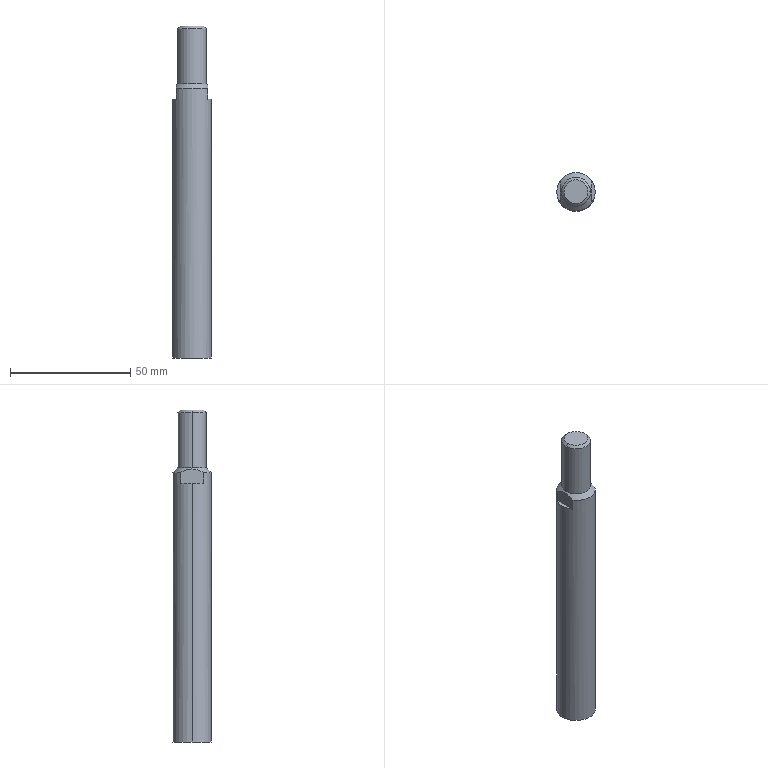Part | STEP file | 1 solid | 14 faces | box 16 x 16 x 138 mm | volume 25426 mm3 | plane 6 | cylinder 4 | cone 4 | commonest cylinder face diameters 12 x2 16 x2
STEP:
#1=CARTESIAN_POINT('',(8.,0.,-84.));
#2=VERTEX_POINT('',#1);
#3=CARTESIAN_POINT('',(-8.,0.,-84.));
#4=VERTEX_POINT('',#3);
#5=CARTESIAN_POINT('',(0.,0.,-84.));
#6=DIRECTION('',(0.,0.,1.));
#7=DIRECTION('',(1.,0.,0.));
#8=AXIS2_PLACEMENT_3D('',#5,#6,#7);
#9=CIRCLE('',#8,8.);
#10=EDGE_CURVE('',#2,#4,#9,.T.);
#11=ORIENTED_EDGE('',*,*,#10,.T.);
#12=CARTESIAN_POINT('',(-8.,0.,23.5));
#13=VERTEX_POINT('',#12);
#14=CARTESIAN_POINT('',(-8.,0.,-84.));
#15=DIRECTION('',(0.,0.,1.));
#16=VECTOR('',#15,1000.);
#17=LINE('',#14,#16);
#18=EDGE_CURVE('',#4,#13,#17,.T.);
#19=ORIENTED_EDGE('',*,*,#18,.T.);
#20=CARTESIAN_POINT('',(-6.5,4.664,23.5));
#21=VERTEX_POINT('',#20);
#22=CARTESIAN_POINT('',(0.,0.,23.5));
#23=DIRECTION('',(0.,0.,1.));
#24=DIRECTION('',(1.,0.,0.));
#25=AXIS2_PLACEMENT_3D('',#22,#23,#24);
#26=CIRCLE('',#25,8.);
#27=EDGE_CURVE('',#21,#13,#26,.T.);
#28=ORIENTED_EDGE('',*,*,#27,.F.);
#29=CARTESIAN_POINT('',(-6.5,4.664,28.));
#30=VERTEX_POINT('',#29);
#31=CARTESIAN_POINT('',(-6.5,4.664,-84.));
#32=DIRECTION('',(0.,0.,1.));
#33=VECTOR('',#32,1000.);
#34=LINE('',#31,#33);
#35=EDGE_CURVE('',#21,#30,#34,.T.);
#36=ORIENTED_EDGE('',*,*,#35,.T.);
#37=CARTESIAN_POINT('',(6.5,4.664,28.));
#38=VERTEX_POINT('',#37);
#39=CARTESIAN_POINT('',(0.,0.,28.));
#40=DIRECTION('',(0.,0.,1.));
#41=DIRECTION('',(1.,0.,0.));
#42=AXIS2_PLACEMENT_3D('',#39,#40,#41);
#43=CIRCLE('',#42,8.);
#44=EDGE_CURVE('',#38,#30,#43,.T.);
#45=ORIENTED_EDGE('',*,*,#44,.F.);
#46=CARTESIAN_POINT('',(6.5,4.664,23.5));
#47=VERTEX_POINT('',#46);
#48=CARTESIAN_POINT('',(6.5,4.664,-84.));
#49=DIRECTION('',(0.,0.,-1.));
#50=VECTOR('',#49,1000.);
#51=LINE('',#48,#50);
#52=EDGE_CURVE('',#38,#47,#51,.T.);
#53=ORIENTED_EDGE('',*,*,#52,.T.);
#54=CARTESIAN_POINT('',(8.,0.,23.5));
#55=VERTEX_POINT('',#54);
#56=CARTESIAN_POINT('',(0.,0.,23.5));
#57=DIRECTION('',(0.,0.,1.));
#58=DIRECTION('',(1.,0.,0.));
#59=AXIS2_PLACEMENT_3D('',#56,#57,#58);
#60=CIRCLE('',#59,8.);
#61=EDGE_CURVE('',#55,#47,#60,.T.);
#62=ORIENTED_EDGE('',*,*,#61,.F.);
#63=CARTESIAN_POINT('',(8.,0.,-84.));
#64=DIRECTION('',(0.,0.,1.));
#65=VECTOR('',#64,1000.);
#66=LINE('',#63,#65);
#67=EDGE_CURVE('',#2,#55,#66,.T.);
#68=ORIENTED_EDGE('',*,*,#67,.F.);
#69=EDGE_LOOP('',(#11,#19,#28,#36,#45,#53,#62,#68));
#70=FACE_OUTER_BOUND('',#69,.T.);
#71=CARTESIAN_POINT('',(0.,0.,-84.));
#72=DIRECTION('',(0.,0.,1.));
#73=DIRECTION('',(1.,0.,0.));
#74=AXIS2_PLACEMENT_3D('',#71,#72,#73);
#75=CYLINDRICAL_SURFACE('',#74,8.);
#76=ADVANCED_FACE('',(#70),#75,.T.);
#77=CARTESIAN_POINT('',(6.,0.,30.));
#78=VERTEX_POINT('',#77);
#79=CARTESIAN_POINT('',(-6.,0.,30.));
#80=VERTEX_POINT('',#79);
#81=CARTESIAN_POINT('',(0.,0.,30.));
#82=DIRECTION('',(0.,0.,1.));
#83=DIRECTION('',(1.,0.,0.));
#84=AXIS2_PLACEMENT_3D('',#81,#82,#83);
#85=CIRCLE('',#84,6.);
#86=EDGE_CURVE('',#78,#80,#85,.T.);
#87=ORIENTED_EDGE('',*,*,#86,.F.);
#88=CARTESIAN_POINT('',(6.5,0.,29.5));
#89=VERTEX_POINT('',#88);
#90=CARTESIAN_POINT('',(8.,0.,28.));
#91=DIRECTION('',(0.7071,0.,-0.7071));
#92=VECTOR('',#91,1000.);
#93=LINE('',#90,#92);
#94=EDGE_CURVE('',#78,#89,#93,.T.);
#95=ORIENTED_EDGE('',*,*,#94,.T.);
#96=CARTESIAN_POINT('',(6.5,0.,29.5));
#97=CARTESIAN_POINT('',(6.5,0.2071,29.5));
#98=CARTESIAN_POINT('',(6.5,0.4165,29.49));
#99=CARTESIAN_POINT('',(6.5,0.8304,29.45));
#100=CARTESIAN_POINT('',(6.5,1.035,29.421));
#101=CARTESIAN_POINT('',(6.5,1.644,29.307));
#102=CARTESIAN_POINT('',(6.5,2.042,29.197));
#103=CARTESIAN_POINT('',(6.5,2.825,28.922));
#104=CARTESIAN_POINT('',(6.5,3.208,28.759));
#105=CARTESIAN_POINT('',(6.5,3.949,28.401));
#106=CARTESIAN_POINT('',(6.5,4.31,28.206));
#107=CARTESIAN_POINT('',(6.5,4.664,28.));
#108=B_SPLINE_CURVE_WITH_KNOTS('',3,(#96,#97,#98,#99,#100,#101,#102,#103,#104,#105,#106,#107),.UNSPECIFIED.,.F.,.F.,(4,2,2,2,2,4),(0.01525,0.01587,0.01649,0.01772,0.01896,0.02019),.UNSPECIFIED.);
#109=EDGE_CURVE('',#89,#38,#108,.T.);
#110=ORIENTED_EDGE('',*,*,#109,.T.);
#111=ORIENTED_EDGE('',*,*,#44,.T.);
#112=CARTESIAN_POINT('',(-6.5,0.,29.5));
#113=VERTEX_POINT('',#112);
#114=CARTESIAN_POINT('',(-6.5,4.664,28.));
#115=CARTESIAN_POINT('',(-6.5,4.31,28.206));
#116=CARTESIAN_POINT('',(-6.5,3.949,28.401));
#117=CARTESIAN_POINT('',(-6.5,3.208,28.759));
#118=CARTESIAN_POINT('',(-6.5,2.825,28.922));
#119=CARTESIAN_POINT('',(-6.5,2.042,29.197));
#120=CARTESIAN_POINT('',(-6.5,1.644,29.307));
#121=CARTESIAN_POINT('',(-6.5,1.035,29.421));
#122=CARTESIAN_POINT('',(-6.5,0.8304,29.45));
#123=CARTESIAN_POINT('',(-6.5,0.4165,29.49));
#124=CARTESIAN_POINT('',(-6.5,0.2071,29.5));
#125=CARTESIAN_POINT('',(-6.5,0.,29.5));
#126=B_SPLINE_CURVE_WITH_KNOTS('',3,(#114,#115,#116,#117,#118,#119,#120,#121,#122,#123,#124,#125),.UNSPECIFIED.,.F.,.F.,(4,2,2,2,2,4),(0.003921,0.005149,0.006377,0.007605,0.008219,0.008834),.UNSPECIFIED.);
#127=EDGE_CURVE('',#30,#113,#126,.T.);
#128=ORIENTED_EDGE('',*,*,#127,.T.);
#129=CARTESIAN_POINT('',(-8.,0.,28.));
#130=DIRECTION('',(-0.7071,0.,-0.7071));
#131=VECTOR('',#130,1000.);
#132=LINE('',#129,#131);
#133=EDGE_CURVE('',#80,#113,#132,.T.);
#134=ORIENTED_EDGE('',*,*,#133,.F.);
#135=EDGE_LOOP('',(#87,#95,#110,#111,#128,#134));
#136=FACE_OUTER_BOUND('',#135,.T.);
#137=CARTESIAN_POINT('',(0.,0.,28.));
#138=DIRECTION('',(0.,0.,-1.));
#139=DIRECTION('',(-1.,0.,0.));
#140=AXIS2_PLACEMENT_3D('',#137,#138,#139);
#141=CONICAL_SURFACE('',#140,8.,0.7854);
#142=ADVANCED_FACE('',(#136),#141,.T.);
#143=ORIENTED_EDGE('',*,*,#86,.T.);
#144=CARTESIAN_POINT('',(-6.,0.,52.927));
#145=VERTEX_POINT('',#144);
#146=CARTESIAN_POINT('',(-6.,0.,-84.));
#147=DIRECTION('',(0.,0.,1.));
#148=VECTOR('',#147,1000.);
#149=LINE('',#146,#148);
#150=EDGE_CURVE('',#80,#145,#149,.T.);
#151=ORIENTED_EDGE('',*,*,#150,.T.);
#152=CARTESIAN_POINT('',(6.,0.,52.927));
#153=VERTEX_POINT('',#152);
#154=CARTESIAN_POINT('',(0.,0.,52.927));
#155=DIRECTION('',(0.,0.,1.));
#156=DIRECTION('',(1.,0.,0.));
#157=AXIS2_PLACEMENT_3D('',#154,#155,#156);
#158=CIRCLE('',#157,6.);
#159=EDGE_CURVE('',#153,#145,#158,.T.);
#160=ORIENTED_EDGE('',*,*,#159,.F.);
#161=CARTESIAN_POINT('',(6.,0.,-84.));
#162=DIRECTION('',(0.,0.,1.));
#163=VECTOR('',#162,1000.);
#164=LINE('',#161,#163);
#165=EDGE_CURVE('',#78,#153,#164,.T.);
#166=ORIENTED_EDGE('',*,*,#165,.F.);
#167=EDGE_LOOP('',(#143,#151,#160,#166));
#168=FACE_OUTER_BOUND('',#167,.T.);
#169=CARTESIAN_POINT('',(0.,0.,-84.));
#170=DIRECTION('',(0.,0.,1.));
#171=DIRECTION('',(1.,0.,0.));
#172=AXIS2_PLACEMENT_3D('',#169,#170,#171);
#173=CYLINDRICAL_SURFACE('',#172,6.);
#174=ADVANCED_FACE('',(#168),#173,.T.);
#175=CARTESIAN_POINT('',(4.926,0.,54.));
#176=VERTEX_POINT('',#175);
#177=CARTESIAN_POINT('',(-4.926,0.,54.));
#178=VERTEX_POINT('',#177);
#179=CARTESIAN_POINT('',(0.,0.,54.));
#180=DIRECTION('',(0.,0.,1.));
#181=DIRECTION('',(1.,0.,0.));
#182=AXIS2_PLACEMENT_3D('',#179,#180,#181);
#183=CIRCLE('',#182,4.926);
#184=EDGE_CURVE('',#176,#178,#183,.T.);
#185=ORIENTED_EDGE('',*,*,#184,.F.);
#186=CARTESIAN_POINT('',(6.,0.,52.927));
#187=DIRECTION('',(0.7071,0.,-0.7071));
#188=VECTOR('',#187,1000.);
#189=LINE('',#186,#188);
#190=EDGE_CURVE('',#176,#153,#189,.T.);
#191=ORIENTED_EDGE('',*,*,#190,.T.);
#192=ORIENTED_EDGE('',*,*,#159,.T.);
#193=CARTESIAN_POINT('',(-6.,0.,52.927));
#194=DIRECTION('',(-0.7071,0.,-0.7071));
#195=VECTOR('',#194,1000.);
#196=LINE('',#193,#195);
#197=EDGE_CURVE('',#178,#145,#196,.T.);
#198=ORIENTED_EDGE('',*,*,#197,.F.);
#199=EDGE_LOOP('',(#185,#191,#192,#198));
#200=FACE_OUTER_BOUND('',#199,.T.);
#201=CARTESIAN_POINT('',(0.,0.,52.927));
#202=DIRECTION('',(0.,0.,-1.));
#203=DIRECTION('',(-1.,0.,0.));
#204=AXIS2_PLACEMENT_3D('',#201,#202,#203);
#205=CONICAL_SURFACE('',#204,6.,0.7854);
#206=ADVANCED_FACE('',(#200),#205,.T.);
#207=CARTESIAN_POINT('',(0.,0.,54.));
#208=DIRECTION('',(0.,0.,1.));
#209=DIRECTION('',(1.,0.,0.));
#210=AXIS2_PLACEMENT_3D('',#207,#208,#209);
#211=CIRCLE('',#210,4.926);
#212=EDGE_CURVE('',#178,#176,#211,.T.);
#213=ORIENTED_EDGE('',*,*,#212,.T.);
#214=ORIENTED_EDGE('',*,*,#184,.T.);
#215=EDGE_LOOP('',(#213,#214));
#216=FACE_OUTER_BOUND('',#215,.T.);
#217=CARTESIAN_POINT('',(0.,0.,54.));
#218=DIRECTION('',(0.,0.,-1.));
#219=DIRECTION('',(-1.,0.,0.));
#220=AXIS2_PLACEMENT_3D('',#217,#218,#219);
#221=PLANE('',#220);
#222=ADVANCED_FACE('',(#216),#221,.F.);
#223=ORIENTED_EDGE('',*,*,#190,.F.);
#224=ORIENTED_EDGE('',*,*,#212,.F.);
#225=ORIENTED_EDGE('',*,*,#197,.T.);
#226=CARTESIAN_POINT('',(0.,0.,52.927));
#227=DIRECTION('',(0.,0.,1.));
#228=DIRECTION('',(1.,0.,0.));
#229=AXIS2_PLACEMENT_3D('',#226,#227,#228);
#230=CIRCLE('',#229,6.);
#231=EDGE_CURVE('',#145,#153,#230,.T.);
#232=ORIENTED_EDGE('',*,*,#231,.T.);
#233=EDGE_LOOP('',(#223,#224,#225,#232));
#234=FACE_OUTER_BOUND('',#233,.T.);
#235=CARTESIAN_POINT('',(0.,0.,52.927));
#236=DIRECTION('',(0.,0.,-1.));
#237=DIRECTION('',(-1.,0.,0.));
#238=AXIS2_PLACEMENT_3D('',#235,#236,#237);
#239=CONICAL_SURFACE('',#238,6.,0.7854);
#240=ADVANCED_FACE('',(#234),#239,.T.);
#241=ORIENTED_EDGE('',*,*,#150,.F.);
#242=CARTESIAN_POINT('',(0.,0.,30.));
#243=DIRECTION('',(0.,0.,1.));
#244=DIRECTION('',(1.,0.,0.));
#245=AXIS2_PLACEMENT_3D('',#242,#243,#244);
#246=CIRCLE('',#245,6.);
#247=EDGE_CURVE('',#80,#78,#246,.T.);
#248=ORIENTED_EDGE('',*,*,#247,.T.);
#249=ORIENTED_EDGE('',*,*,#165,.T.);
#250=ORIENTED_EDGE('',*,*,#231,.F.);
#251=EDGE_LOOP('',(#241,#248,#249,#250));
#252=FACE_OUTER_BOUND('',#251,.T.);
#253=CARTESIAN_POINT('',(0.,0.,-84.));
#254=DIRECTION('',(0.,0.,1.));
#255=DIRECTION('',(1.,0.,0.));
#256=AXIS2_PLACEMENT_3D('',#253,#254,#255);
#257=CYLINDRICAL_SURFACE('',#256,6.);
#258=ADVANCED_FACE('',(#252),#257,.T.);
#259=ORIENTED_EDGE('',*,*,#94,.F.);
#260=ORIENTED_EDGE('',*,*,#247,.F.);
#261=ORIENTED_EDGE('',*,*,#133,.T.);
#262=CARTESIAN_POINT('',(-6.5,-4.664,28.));
#263=VERTEX_POINT('',#262);
#264=CARTESIAN_POINT('',(-6.5,0.,29.5));
#265=CARTESIAN_POINT('',(-6.5,-0.4145,29.5));
#266=CARTESIAN_POINT('',(-6.5,-0.8244,29.46));
#267=CARTESIAN_POINT('',(-6.5,-1.636,29.309));
#268=CARTESIAN_POINT('',(-6.5,-2.04,29.197));
#269=CARTESIAN_POINT('',(-6.5,-3.213,28.786));
#270=CARTESIAN_POINT('',(-6.5,-3.949,28.417));
#271=CARTESIAN_POINT('',(-6.5,-4.664,28.));
#272=B_SPLINE_CURVE_WITH_KNOTS('',3,(#264,#265,#266,#267,#268,#269,#270,#271),.UNSPECIFIED.,.F.,.F.,(4,2,2,4),(0.008834,0.01006,0.01129,0.01375),.UNSPECIFIED.);
#273=EDGE_CURVE('',#113,#263,#272,.T.);
#274=ORIENTED_EDGE('',*,*,#273,.T.);
#275=CARTESIAN_POINT('',(6.5,-4.664,28.));
#276=VERTEX_POINT('',#275);
#277=CARTESIAN_POINT('',(0.,0.,28.));
#278=DIRECTION('',(0.,0.,1.));
#279=DIRECTION('',(1.,0.,0.));
#280=AXIS2_PLACEMENT_3D('',#277,#278,#279);
#281=CIRCLE('',#280,8.);
#282=EDGE_CURVE('',#263,#276,#281,.T.);
#283=ORIENTED_EDGE('',*,*,#282,.T.);
#284=CARTESIAN_POINT('',(6.5,-4.664,28.));
#285=CARTESIAN_POINT('',(6.5,-3.949,28.417));
#286=CARTESIAN_POINT('',(6.5,-3.213,28.786));
#287=CARTESIAN_POINT('',(6.5,-2.04,29.197));
#288=CARTESIAN_POINT('',(6.5,-1.636,29.309));
#289=CARTESIAN_POINT('',(6.5,-0.8244,29.46));
#290=CARTESIAN_POINT('',(6.5,-0.4145,29.5));
#291=CARTESIAN_POINT('',(6.5,0.,29.5));
#292=B_SPLINE_CURVE_WITH_KNOTS('',3,(#284,#285,#286,#287,#288,#289,#290,#291),.UNSPECIFIED.,.F.,.F.,(4,2,2,4),(0.01031,0.01278,0.01402,0.01525),.UNSPECIFIED.);
#293=EDGE_CURVE('',#276,#89,#292,.T.);
#294=ORIENTED_EDGE('',*,*,#293,.T.);
#295=EDGE_LOOP('',(#259,#260,#261,#274,#283,#294));
#296=FACE_OUTER_BOUND('',#295,.T.);
#297=CARTESIAN_POINT('',(0.,0.,28.));
#298=DIRECTION('',(0.,0.,-1.));
#299=DIRECTION('',(-1.,0.,0.));
#300=AXIS2_PLACEMENT_3D('',#297,#298,#299);
#301=CONICAL_SURFACE('',#300,8.,0.7854);
#302=ADVANCED_FACE('',(#296),#301,.T.);
#303=ORIENTED_EDGE('',*,*,#18,.F.);
#304=CARTESIAN_POINT('',(0.,0.,-84.));
#305=DIRECTION('',(0.,0.,1.));
#306=DIRECTION('',(1.,0.,0.));
#307=AXIS2_PLACEMENT_3D('',#304,#305,#306);
#308=CIRCLE('',#307,8.);
#309=EDGE_CURVE('',#4,#2,#308,.T.);
#310=ORIENTED_EDGE('',*,*,#309,.T.);
#311=ORIENTED_EDGE('',*,*,#67,.T.);
#312=CARTESIAN_POINT('',(6.5,-4.664,23.5));
#313=VERTEX_POINT('',#312);
#314=CARTESIAN_POINT('',(0.,0.,23.5));
#315=DIRECTION('',(0.,0.,1.));
#316=DIRECTION('',(1.,0.,0.));
#317=AXIS2_PLACEMENT_3D('',#314,#315,#316);
#318=CIRCLE('',#317,8.);
#319=EDGE_CURVE('',#313,#55,#318,.T.);
#320=ORIENTED_EDGE('',*,*,#319,.F.);
#321=CARTESIAN_POINT('',(6.5,-4.664,-84.));
#322=DIRECTION('',(0.,0.,1.));
#323=VECTOR('',#322,1000.);
#324=LINE('',#321,#323);
#325=EDGE_CURVE('',#313,#276,#324,.T.);
#326=ORIENTED_EDGE('',*,*,#325,.T.);
#327=ORIENTED_EDGE('',*,*,#282,.F.);
#328=CARTESIAN_POINT('',(-6.5,-4.664,23.5));
#329=VERTEX_POINT('',#328);
#330=CARTESIAN_POINT('',(-6.5,-4.664,-84.));
#331=DIRECTION('',(0.,0.,-1.));
#332=VECTOR('',#331,1000.);
#333=LINE('',#330,#332);
#334=EDGE_CURVE('',#263,#329,#333,.T.);
#335=ORIENTED_EDGE('',*,*,#334,.T.);
#336=CARTESIAN_POINT('',(0.,0.,23.5));
#337=DIRECTION('',(0.,0.,1.));
#338=DIRECTION('',(1.,0.,0.));
#339=AXIS2_PLACEMENT_3D('',#336,#337,#338);
#340=CIRCLE('',#339,8.);
#341=EDGE_CURVE('',#13,#329,#340,.T.);
#342=ORIENTED_EDGE('',*,*,#341,.F.);
#343=EDGE_LOOP('',(#303,#310,#311,#320,#326,#327,#335,#342));
#344=FACE_OUTER_BOUND('',#343,.T.);
#345=CARTESIAN_POINT('',(0.,0.,-84.));
#346=DIRECTION('',(0.,0.,1.));
#347=DIRECTION('',(1.,0.,0.));
#348=AXIS2_PLACEMENT_3D('',#345,#346,#347);
#349=CYLINDRICAL_SURFACE('',#348,8.);
#350=ADVANCED_FACE('',(#344),#349,.T.);
#351=ORIENTED_EDGE('',*,*,#10,.F.);
#352=ORIENTED_EDGE('',*,*,#309,.F.);
#353=EDGE_LOOP('',(#351,#352));
#354=FACE_OUTER_BOUND('',#353,.T.);
#355=CARTESIAN_POINT('',(0.,8.,-84.));
#356=DIRECTION('',(0.,0.,1.));
#357=DIRECTION('',(1.,0.,0.));
#358=AXIS2_PLACEMENT_3D('',#355,#356,#357);
#359=PLANE('',#358);
#360=ADVANCED_FACE('',(#354),#359,.F.);
#361=ORIENTED_EDGE('',*,*,#319,.T.);
#362=ORIENTED_EDGE('',*,*,#61,.T.);
#363=CARTESIAN_POINT('',(6.5,17.5,23.5));
#364=DIRECTION('',(0.,-1.,0.));
#365=VECTOR('',#364,1000.);
#366=LINE('',#363,#365);
#367=EDGE_CURVE('',#47,#313,#366,.T.);
#368=ORIENTED_EDGE('',*,*,#367,.T.);
#369=EDGE_LOOP('',(#361,#362,#368));
#370=FACE_OUTER_BOUND('',#369,.T.);
#371=CARTESIAN_POINT('',(-16.5,-17.5,23.5));
#372=DIRECTION('',(0.,0.,1.));
#373=DIRECTION('',(1.,0.,0.));
#374=AXIS2_PLACEMENT_3D('',#371,#372,#373);
#375=PLANE('',#374);
#376=ADVANCED_FACE('',(#370),#375,.T.);
#377=ORIENTED_EDGE('',*,*,#367,.F.);
#378=ORIENTED_EDGE('',*,*,#52,.F.);
#379=ORIENTED_EDGE('',*,*,#109,.F.);
#380=ORIENTED_EDGE('',*,*,#293,.F.);
#381=ORIENTED_EDGE('',*,*,#325,.F.);
#382=EDGE_LOOP('',(#377,#378,#379,#380,#381));
#383=FACE_OUTER_BOUND('',#382,.T.);
#384=CARTESIAN_POINT('',(6.5,17.5,23.5));
#385=DIRECTION('',(-1.,0.,0.));
#386=DIRECTION('',(0.,0.,1.));
#387=AXIS2_PLACEMENT_3D('',#384,#385,#386);
#388=PLANE('',#387);
#389=ADVANCED_FACE('',(#383),#388,.F.);
#390=CARTESIAN_POINT('',(-6.5,-17.5,23.5));
#391=DIRECTION('',(0.,1.,0.));
#392=VECTOR('',#391,1000.);
#393=LINE('',#390,#392);
#394=EDGE_CURVE('',#329,#21,#393,.T.);
#395=ORIENTED_EDGE('',*,*,#394,.F.);
#396=ORIENTED_EDGE('',*,*,#334,.F.);
#397=ORIENTED_EDGE('',*,*,#273,.F.);
#398=ORIENTED_EDGE('',*,*,#127,.F.);
#399=ORIENTED_EDGE('',*,*,#35,.F.);
#400=EDGE_LOOP('',(#395,#396,#397,#398,#399));
#401=FACE_OUTER_BOUND('',#400,.T.);
#402=CARTESIAN_POINT('',(-6.5,-17.5,23.5));
#403=DIRECTION('',(1.,0.,0.));
#404=DIRECTION('',(0.,0.,-1.));
#405=AXIS2_PLACEMENT_3D('',#402,#403,#404);
#406=PLANE('',#405);
#407=ADVANCED_FACE('',(#401),#406,.F.);
#408=ORIENTED_EDGE('',*,*,#27,.T.);
#409=ORIENTED_EDGE('',*,*,#341,.T.);
#410=ORIENTED_EDGE('',*,*,#394,.T.);
#411=EDGE_LOOP('',(#408,#409,#410));
#412=FACE_OUTER_BOUND('',#411,.T.);
#413=CARTESIAN_POINT('',(-16.5,-17.5,23.5));
#414=DIRECTION('',(0.,0.,1.));
#415=DIRECTION('',(1.,0.,0.));
#416=AXIS2_PLACEMENT_3D('',#413,#414,#415);
#417=PLANE('',#416);
#418=ADVANCED_FACE('',(#412),#417,.T.);
#419=CLOSED_SHELL('',(#76,#142,#174,#206,#222,#240,#258,#302,#350,#360,#376,#389,#407,#418));
#420=MANIFOLD_SOLID_BREP('',#419);
#421=CARTESIAN_POINT('',(0.,0.,0.));
#422=DIRECTION('',(0.,0.,1.));
#423=DIRECTION('',(1.,0.,0.));
#424=AXIS2_PLACEMENT_3D('',#421,#422,#423);
#425=(LENGTH_UNIT()NAMED_UNIT(*)SI_UNIT(.MILLI.,.METRE.));
#426=UNCERTAINTY_MEASURE_WITH_UNIT(LENGTH_MEASURE(0.00001),#425,'','');
#427=(NAMED_UNIT(*)PLANE_ANGLE_UNIT()SI_UNIT($,.RADIAN.));
#428=(NAMED_UNIT(*)SI_UNIT($,.STERADIAN.)SOLID_ANGLE_UNIT());
#429=(GEOMETRIC_REPRESENTATION_CONTEXT(3)GLOBAL_UNCERTAINTY_ASSIGNED_CONTEXT((#426))GLOBAL_UNIT_ASSIGNED_CONTEXT((#425,#427,#428))REPRESENTATION_CONTEXT('',''));
#430=ADVANCED_BREP_SHAPE_REPRESENTATION('',(#420,#424),#429);